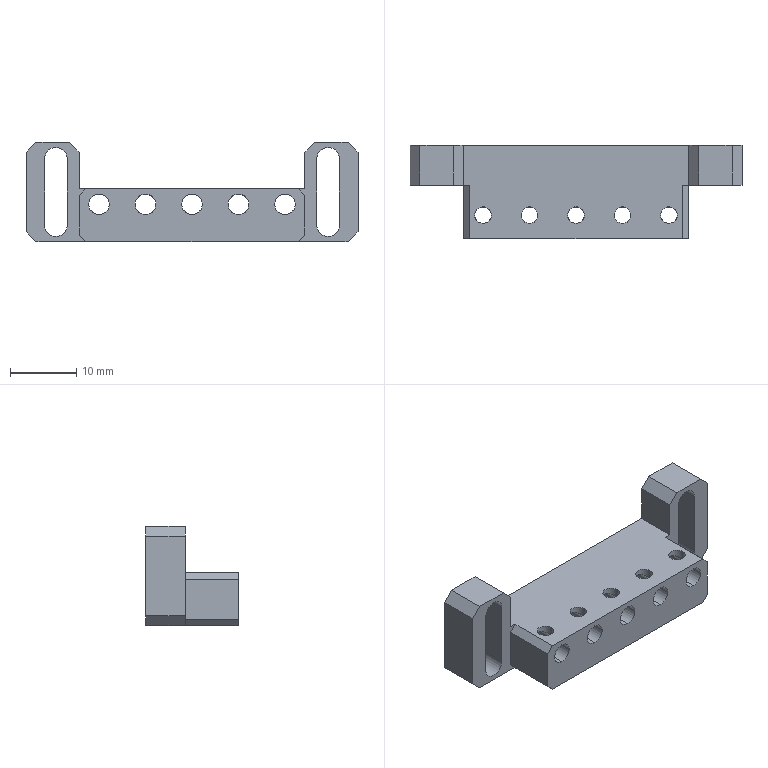Part | STEP file | 10000020473swp000-1 | 1 solid | 64 faces | box 50 x 14 x 15 mm | volume 4019 mm3 | cylinder 36 | plane 28 | commonest cylinder face diameters 2.5 x20 3.1 x10 3.4 x6